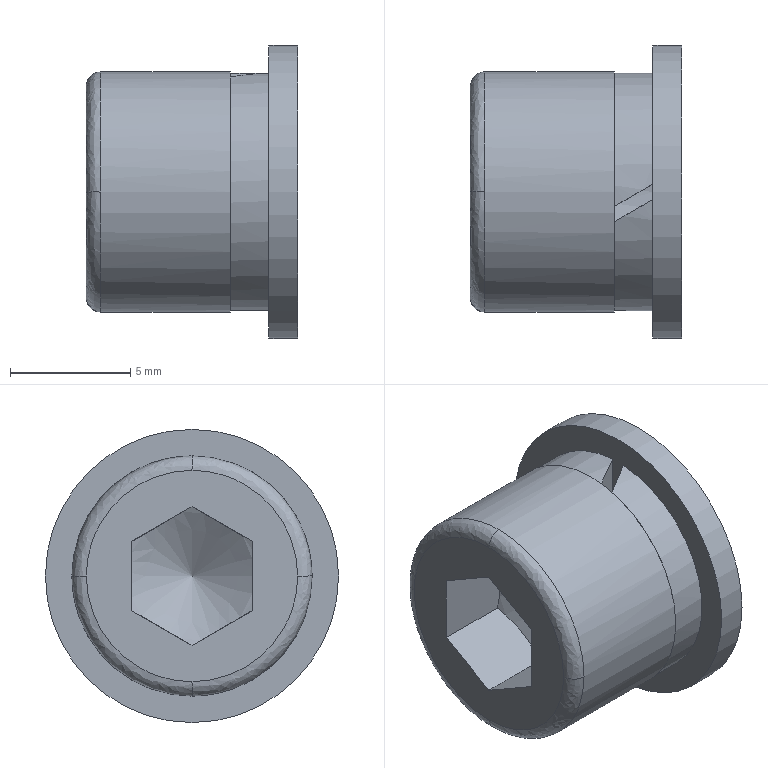Part | NX | features BREP 2 | 2 solids | 23 faces | box 8.8 x 12.2 x 12.2 mm | volume 563.29 mm3 | plane 13 | cylinder 5 | spline 4 | cone 1 | commonest cylinder face diameters 6.1 x1 6.5 x1 9.9 x1 10 x1 12.2 x1
STEP:
#1=CARTESIAN_POINT('',(96.982,177.189,-1.445));
#2=VERTEX_POINT('',#1);
#3=CARTESIAN_POINT('',(96.982,177.189,1.445));
#4=VERTEX_POINT('',#3);
#5=CARTESIAN_POINT('',(96.982,177.189,-1.445));
#6=CARTESIAN_POINT('',(97.255,177.189,-0.5008));
#7=CARTESIAN_POINT('',(97.255,177.189,0.5008));
#8=CARTESIAN_POINT('',(96.982,177.189,1.445));
#9=B_SPLINE_CURVE_WITH_KNOTS('',3,(#5,#6,#7,#8),.UNSPECIFIED.,.F.,.F.,(4,4),(0.,0.002924),.UNSPECIFIED.);
#10=EDGE_CURVE('',#2,#4,#9,.T.);
#11=ORIENTED_EDGE('',*,*,#10,.T.);
#12=CARTESIAN_POINT('',(96.982,179.689,2.887));
#13=VERTEX_POINT('',#12);
#14=CARTESIAN_POINT('',(96.982,177.189,1.445));
#15=CARTESIAN_POINT('',(97.254,178.005,1.916));
#16=CARTESIAN_POINT('',(97.254,178.872,2.416));
#17=CARTESIAN_POINT('',(96.982,179.689,2.887));
#18=B_SPLINE_CURVE_WITH_KNOTS('',3,(#14,#15,#16,#17),.UNSPECIFIED.,.F.,.F.,(4,4),(0.,0.002915),.UNSPECIFIED.);
#19=EDGE_CURVE('',#4,#13,#18,.T.);
#20=ORIENTED_EDGE('',*,*,#19,.T.);
#21=CARTESIAN_POINT('',(96.982,182.189,1.445));
#22=VERTEX_POINT('',#21);
#23=CARTESIAN_POINT('',(96.982,179.689,2.887));
#24=CARTESIAN_POINT('',(97.254,180.505,2.416));
#25=CARTESIAN_POINT('',(97.254,181.372,1.917));
#26=CARTESIAN_POINT('',(96.982,182.189,1.445));
#27=B_SPLINE_CURVE_WITH_KNOTS('',3,(#23,#24,#25,#26),.UNSPECIFIED.,.F.,.F.,(4,4),(0.,0.002915),.UNSPECIFIED.);
#28=EDGE_CURVE('',#13,#22,#27,.T.);
#29=ORIENTED_EDGE('',*,*,#28,.T.);
#30=CARTESIAN_POINT('',(96.982,182.189,-1.445));
#31=VERTEX_POINT('',#30);
#32=CARTESIAN_POINT('',(96.982,182.189,1.445));
#33=CARTESIAN_POINT('',(97.255,182.189,0.5008));
#34=CARTESIAN_POINT('',(97.255,182.189,-0.5008));
#35=CARTESIAN_POINT('',(96.982,182.189,-1.445));
#36=B_SPLINE_CURVE_WITH_KNOTS('',3,(#32,#33,#34,#35),.UNSPECIFIED.,.F.,.F.,(4,4),(0.,0.002924),.UNSPECIFIED.);
#37=EDGE_CURVE('',#22,#31,#36,.T.);
#38=ORIENTED_EDGE('',*,*,#37,.T.);
#39=CARTESIAN_POINT('',(96.982,179.689,-2.887));
#40=VERTEX_POINT('',#39);
#41=CARTESIAN_POINT('',(96.982,182.189,-1.445));
#42=CARTESIAN_POINT('',(97.254,181.373,-1.916));
#43=CARTESIAN_POINT('',(97.254,180.507,-2.416));
#44=CARTESIAN_POINT('',(96.982,179.689,-2.887));
#45=B_SPLINE_CURVE_WITH_KNOTS('',3,(#41,#42,#43,#44),.UNSPECIFIED.,.F.,.F.,(4,4),(0.,0.002915),.UNSPECIFIED.);
#46=EDGE_CURVE('',#31,#40,#45,.T.);
#47=ORIENTED_EDGE('',*,*,#46,.T.);
#48=CARTESIAN_POINT('',(96.982,179.689,-2.887));
#49=CARTESIAN_POINT('',(97.254,178.873,-2.416));
#50=CARTESIAN_POINT('',(97.254,178.007,-1.917));
#51=CARTESIAN_POINT('',(96.982,177.189,-1.445));
#52=B_SPLINE_CURVE_WITH_KNOTS('',3,(#48,#49,#50,#51),.UNSPECIFIED.,.F.,.F.,(4,4),(0.,0.002915),.UNSPECIFIED.);
#53=EDGE_CURVE('',#40,#2,#52,.T.);
#54=ORIENTED_EDGE('',*,*,#53,.T.);
#55=EDGE_LOOP('',(#11,#20,#29,#38,#47,#54));
#56=FACE_BOUND('',#55,.T.);
#57=CARTESIAN_POINT('',(98.649,179.689,0.));
#58=VERTEX_POINT('',#57);
#59=VERTEX_LOOP('',#58);
#60=FACE_BOUND('',#59,.T.);
#61=CARTESIAN_POINT('',(97.816,179.689,0.));
#62=DIRECTION('',(-1.,0.,0.));
#63=DIRECTION('',(0.,-1.,0.));
#64=AXIS2_PLACEMENT_3D('',#61,#62,#63);
#65=CONICAL_SURFACE('',#64,1.444,1.047);
#66=ADVANCED_FACE('',(#56,#60),#65,.F.);
#67=ORIENTED_EDGE('',*,*,#37,.F.);
#68=CARTESIAN_POINT('',(93.982,182.189,1.445));
#69=VERTEX_POINT('',#68);
#70=CARTESIAN_POINT('',(93.982,182.189,1.445));
#71=DIRECTION('',(1.,0.,0.));
#72=VECTOR('',#71,1000.);
#73=LINE('',#70,#72);
#74=EDGE_CURVE('',#69,#22,#73,.T.);
#75=ORIENTED_EDGE('',*,*,#74,.F.);
#76=CARTESIAN_POINT('',(93.982,182.189,-1.445));
#77=VERTEX_POINT('',#76);
#78=CARTESIAN_POINT('',(93.982,182.189,0.));
#79=DIRECTION('',(0.,0.,1.));
#80=VECTOR('',#79,1000.);
#81=LINE('',#78,#80);
#82=EDGE_CURVE('',#77,#69,#81,.T.);
#83=ORIENTED_EDGE('',*,*,#82,.F.);
#84=CARTESIAN_POINT('',(93.982,182.189,-1.445));
#85=DIRECTION('',(1.,0.,0.));
#86=VECTOR('',#85,1000.);
#87=LINE('',#84,#86);
#88=EDGE_CURVE('',#77,#31,#87,.T.);
#89=ORIENTED_EDGE('',*,*,#88,.T.);
#90=EDGE_LOOP('',(#67,#75,#83,#89));
#91=FACE_BOUND('',#90,.T.);
#92=CARTESIAN_POINT('',(93.982,182.189,-1.445));
#93=DIRECTION('',(0.,-1.,0.));
#94=DIRECTION('',(0.,0.,-1.));
#95=AXIS2_PLACEMENT_3D('',#92,#93,#94);
#96=PLANE('',#95);
#97=ADVANCED_FACE('',(#91),#96,.T.);
#98=ORIENTED_EDGE('',*,*,#46,.F.);
#99=ORIENTED_EDGE('',*,*,#88,.F.);
#100=CARTESIAN_POINT('',(93.982,179.689,-2.887));
#101=VERTEX_POINT('',#100);
#102=CARTESIAN_POINT('',(93.982,183.898,-0.4589));
#103=DIRECTION('',(0.,0.8661,0.4998));
#104=VECTOR('',#103,1000.);
#105=LINE('',#102,#104);
#106=EDGE_CURVE('',#101,#77,#105,.T.);
#107=ORIENTED_EDGE('',*,*,#106,.F.);
#108=CARTESIAN_POINT('',(93.982,179.689,-2.887));
#109=DIRECTION('',(-1.,0.,0.));
#110=VECTOR('',#109,1000.);
#111=LINE('',#108,#110);
#112=EDGE_CURVE('',#40,#101,#111,.T.);
#113=ORIENTED_EDGE('',*,*,#112,.F.);
#114=EDGE_LOOP('',(#98,#99,#107,#113));
#115=FACE_BOUND('',#114,.T.);
#116=CARTESIAN_POINT('',(93.982,179.689,-2.888));
#117=DIRECTION('',(0.,-0.4998,0.8661));
#118=DIRECTION('',(1.,0.,0.));
#119=AXIS2_PLACEMENT_3D('',#116,#117,#118);
#120=PLANE('',#119);
#121=ADVANCED_FACE('',(#115),#120,.T.);
#122=ORIENTED_EDGE('',*,*,#53,.F.);
#123=ORIENTED_EDGE('',*,*,#112,.T.);
#124=CARTESIAN_POINT('',(93.982,177.189,-1.445));
#125=VERTEX_POINT('',#124);
#126=CARTESIAN_POINT('',(93.982,181.398,-3.873));
#127=DIRECTION('',(0.,0.8661,-0.4998));
#128=VECTOR('',#127,1000.);
#129=LINE('',#126,#128);
#130=EDGE_CURVE('',#125,#101,#129,.T.);
#131=ORIENTED_EDGE('',*,*,#130,.F.);
#132=CARTESIAN_POINT('',(93.982,177.189,-1.445));
#133=DIRECTION('',(1.,0.,0.));
#134=VECTOR('',#133,1000.);
#135=LINE('',#132,#134);
#136=EDGE_CURVE('',#125,#2,#135,.T.);
#137=ORIENTED_EDGE('',*,*,#136,.T.);
#138=EDGE_LOOP('',(#122,#123,#131,#137));
#139=FACE_BOUND('',#138,.T.);
#140=CARTESIAN_POINT('',(93.982,177.189,-1.445));
#141=DIRECTION('',(0.,0.4998,0.8661));
#142=DIRECTION('',(1.,0.,0.));
#143=AXIS2_PLACEMENT_3D('',#140,#141,#142);
#144=PLANE('',#143);
#145=ADVANCED_FACE('',(#139),#144,.T.);
#146=ORIENTED_EDGE('',*,*,#10,.F.);
#147=ORIENTED_EDGE('',*,*,#136,.F.);
#148=CARTESIAN_POINT('',(93.982,177.189,1.445));
#149=VERTEX_POINT('',#148);
#150=CARTESIAN_POINT('',(93.982,177.189,0.));
#151=DIRECTION('',(0.,0.,-1.));
#152=VECTOR('',#151,1000.);
#153=LINE('',#150,#152);
#154=EDGE_CURVE('',#149,#125,#153,.T.);
#155=ORIENTED_EDGE('',*,*,#154,.F.);
#156=CARTESIAN_POINT('',(93.982,177.189,1.445));
#157=DIRECTION('',(1.,0.,0.));
#158=VECTOR('',#157,1000.);
#159=LINE('',#156,#158);
#160=EDGE_CURVE('',#149,#4,#159,.T.);
#161=ORIENTED_EDGE('',*,*,#160,.T.);
#162=EDGE_LOOP('',(#146,#147,#155,#161));
#163=FACE_BOUND('',#162,.T.);
#164=CARTESIAN_POINT('',(93.982,177.189,1.445));
#165=DIRECTION('',(0.,1.,0.));
#166=DIRECTION('',(0.,0.,1.));
#167=AXIS2_PLACEMENT_3D('',#164,#165,#166);
#168=PLANE('',#167);
#169=ADVANCED_FACE('',(#163),#168,.T.);
#170=ORIENTED_EDGE('',*,*,#19,.F.);
#171=ORIENTED_EDGE('',*,*,#160,.F.);
#172=CARTESIAN_POINT('',(93.982,179.689,2.887));
#173=VERTEX_POINT('',#172);
#174=CARTESIAN_POINT('',(93.982,181.398,3.873));
#175=DIRECTION('',(0.,-0.8661,-0.4998));
#176=VECTOR('',#175,1000.);
#177=LINE('',#174,#176);
#178=EDGE_CURVE('',#173,#149,#177,.T.);
#179=ORIENTED_EDGE('',*,*,#178,.F.);
#180=CARTESIAN_POINT('',(93.982,179.689,2.887));
#181=DIRECTION('',(1.,0.,0.));
#182=VECTOR('',#181,1000.);
#183=LINE('',#180,#182);
#184=EDGE_CURVE('',#173,#13,#183,.T.);
#185=ORIENTED_EDGE('',*,*,#184,.T.);
#186=EDGE_LOOP('',(#170,#171,#179,#185));
#187=FACE_BOUND('',#186,.T.);
#188=CARTESIAN_POINT('',(93.982,179.689,2.888));
#189=DIRECTION('',(0.,0.4998,-0.8661));
#190=DIRECTION('',(-1.,0.,0.));
#191=AXIS2_PLACEMENT_3D('',#188,#189,#190);
#192=PLANE('',#191);
#193=ADVANCED_FACE('',(#187),#192,.T.);
#194=ORIENTED_EDGE('',*,*,#28,.F.);
#195=ORIENTED_EDGE('',*,*,#184,.F.);
#196=CARTESIAN_POINT('',(93.982,183.898,0.4589));
#197=DIRECTION('',(0.,-0.8661,0.4998));
#198=VECTOR('',#197,1000.);
#199=LINE('',#196,#198);
#200=EDGE_CURVE('',#69,#173,#199,.T.);
#201=ORIENTED_EDGE('',*,*,#200,.F.);
#202=ORIENTED_EDGE('',*,*,#74,.T.);
#203=EDGE_LOOP('',(#194,#195,#201,#202));
#204=FACE_BOUND('',#203,.T.);
#205=CARTESIAN_POINT('',(93.982,182.189,1.445));
#206=DIRECTION('',(0.,-0.4998,-0.8661));
#207=DIRECTION('',(-1.,0.,0.));
#208=AXIS2_PLACEMENT_3D('',#205,#206,#207);
#209=PLANE('',#208);
#210=ADVANCED_FACE('',(#204),#209,.T.);
#211=ORIENTED_EDGE('',*,*,#200,.T.);
#212=ORIENTED_EDGE('',*,*,#178,.T.);
#213=ORIENTED_EDGE('',*,*,#154,.T.);
#214=ORIENTED_EDGE('',*,*,#130,.T.);
#215=ORIENTED_EDGE('',*,*,#106,.T.);
#216=ORIENTED_EDGE('',*,*,#82,.T.);
#217=EDGE_LOOP('',(#211,#212,#213,#214,#215,#216));
#218=FACE_BOUND('',#217,.T.);
#219=CARTESIAN_POINT('',(93.982,184.089,0.));
#220=VERTEX_POINT('',#219);
#221=CARTESIAN_POINT('',(93.982,179.689,-4.4));
#222=VERTEX_POINT('',#221);
#223=CARTESIAN_POINT('',(93.982,184.089,0.));
#224=CARTESIAN_POINT('',(93.982,184.089,-1.152));
#225=CARTESIAN_POINT('',(93.982,183.136,-3.446));
#226=CARTESIAN_POINT('',(93.982,180.841,-4.4));
#227=CARTESIAN_POINT('',(93.982,179.689,-4.4));
#228=B_SPLINE_CURVE_WITH_KNOTS('',3,(#223,#224,#225,#226,#227),.UNSPECIFIED.,.F.,.F.,(4,1,4),(0.,4.897,9.794),.UNSPECIFIED.);
#229=EDGE_CURVE('',#220,#222,#228,.T.);
#230=ORIENTED_EDGE('',*,*,#229,.T.);
#231=CARTESIAN_POINT('',(93.982,175.289,0.));
#232=VERTEX_POINT('',#231);
#233=CARTESIAN_POINT('',(93.982,179.689,-4.4));
#234=CARTESIAN_POINT('',(93.982,178.537,-4.4));
#235=CARTESIAN_POINT('',(93.982,176.243,-3.447));
#236=CARTESIAN_POINT('',(93.982,175.289,-1.152));
#237=CARTESIAN_POINT('',(93.982,175.289,0.));
#238=B_SPLINE_CURVE_WITH_KNOTS('',3,(#233,#234,#235,#236,#237),.UNSPECIFIED.,.F.,.F.,(4,1,4),(0.,4.897,9.794),.UNSPECIFIED.);
#239=EDGE_CURVE('',#222,#232,#238,.T.);
#240=ORIENTED_EDGE('',*,*,#239,.T.);
#241=CARTESIAN_POINT('',(93.982,179.689,4.4));
#242=VERTEX_POINT('',#241);
#243=CARTESIAN_POINT('',(93.982,175.289,0.));
#244=CARTESIAN_POINT('',(93.982,175.289,1.152));
#245=CARTESIAN_POINT('',(93.982,176.242,3.446));
#246=CARTESIAN_POINT('',(93.982,178.537,4.4));
#247=CARTESIAN_POINT('',(93.982,179.689,4.4));
#248=B_SPLINE_CURVE_WITH_KNOTS('',3,(#243,#244,#245,#246,#247),.UNSPECIFIED.,.F.,.F.,(4,1,4),(0.,4.896,9.791),.UNSPECIFIED.);
#249=EDGE_CURVE('',#232,#242,#248,.T.);
#250=ORIENTED_EDGE('',*,*,#249,.T.);
#251=CARTESIAN_POINT('',(93.982,179.689,4.4));
#252=CARTESIAN_POINT('',(93.982,180.841,4.4));
#253=CARTESIAN_POINT('',(93.982,183.135,3.447));
#254=CARTESIAN_POINT('',(93.982,184.089,1.152));
#255=CARTESIAN_POINT('',(93.982,184.089,0.));
#256=B_SPLINE_CURVE_WITH_KNOTS('',3,(#251,#252,#253,#254,#255),.UNSPECIFIED.,.F.,.F.,(4,1,4),(0.,4.897,9.794),.UNSPECIFIED.);
#257=EDGE_CURVE('',#242,#220,#256,.T.);
#258=ORIENTED_EDGE('',*,*,#257,.T.);
#259=EDGE_LOOP('',(#230,#240,#250,#258));
#260=FACE_BOUND('',#259,.T.);
#261=CARTESIAN_POINT('',(93.982,183.633,0.));
#262=DIRECTION('',(-1.,0.,0.));
#263=DIRECTION('',(0.,0.,1.));
#264=AXIS2_PLACEMENT_3D('',#261,#262,#263);
#265=PLANE('',#264);
#266=ADVANCED_FACE('',(#218,#260),#265,.T.);
#267=CARTESIAN_POINT('',(94.582,184.689,0.));
#268=VERTEX_POINT('',#267);
#269=CARTESIAN_POINT('',(94.582,179.689,-5.));
#270=VERTEX_POINT('',#269);
#271=CARTESIAN_POINT('',(94.582,179.689,-5.));
#272=CARTESIAN_POINT('',(94.582,180.998,-5.));
#273=CARTESIAN_POINT('',(94.582,183.606,-3.917));
#274=CARTESIAN_POINT('',(94.582,184.689,-1.309));
#275=CARTESIAN_POINT('',(94.582,184.689,0.));
#276=B_SPLINE_CURVE_WITH_KNOTS('',3,(#271,#272,#273,#274,#275),.UNSPECIFIED.,.F.,.F.,(4,1,4),(0.,0.5,1.),.UNSPECIFIED.);
#277=EDGE_CURVE('',#268,#270,#276,.F.);
#278=ORIENTED_EDGE('',*,*,#277,.T.);
#279=CARTESIAN_POINT('',(94.582,179.689,-5.));
#280=CARTESIAN_POINT('',(94.441,179.689,-5.));
#281=CARTESIAN_POINT('',(94.104,179.689,-4.878));
#282=CARTESIAN_POINT('',(93.982,179.689,-4.541));
#283=CARTESIAN_POINT('',(93.982,179.689,-4.4));
#284=B_SPLINE_CURVE_WITH_KNOTS('',3,(#279,#280,#281,#282,#283),.UNSPECIFIED.,.F.,.F.,(4,1,4),(0.,0.6414,1.283),.UNSPECIFIED.);
#285=EDGE_CURVE('',#270,#222,#284,.T.);
#286=ORIENTED_EDGE('',*,*,#285,.T.);
#287=ORIENTED_EDGE('',*,*,#229,.F.);
#288=CARTESIAN_POINT('',(93.982,184.089,0.));
#289=CARTESIAN_POINT('',(93.982,184.23,0.));
#290=CARTESIAN_POINT('',(94.104,184.567,0.));
#291=CARTESIAN_POINT('',(94.441,184.689,0.));
#292=CARTESIAN_POINT('',(94.582,184.689,0.));
#293=B_SPLINE_CURVE_WITH_KNOTS('',3,(#288,#289,#290,#291,#292),.UNSPECIFIED.,.F.,.F.,(4,1,4),(0.,0.6414,1.283),.UNSPECIFIED.);
#294=EDGE_CURVE('',#268,#220,#293,.F.);
#295=ORIENTED_EDGE('',*,*,#294,.F.);
#296=EDGE_LOOP('',(#278,#286,#287,#295));
#297=FACE_BOUND('',#296,.T.);
#298=CARTESIAN_POINT('',(94.582,184.689,0.));
#299=CARTESIAN_POINT('',(94.582,184.689,-5.));
#300=CARTESIAN_POINT('',(94.582,179.689,-5.));
#301=CARTESIAN_POINT('',(93.982,184.689,0.));
#302=CARTESIAN_POINT('',(93.982,184.689,-5.));
#303=CARTESIAN_POINT('',(93.982,179.689,-5.));
#304=CARTESIAN_POINT('',(93.982,184.089,0.));
#305=CARTESIAN_POINT('',(93.982,184.089,-4.4));
#306=CARTESIAN_POINT('',(93.982,179.689,-4.4));
#307=(BOUNDED_SURFACE()B_SPLINE_SURFACE(2,2,((#298,#299,#300),(#301,#302,#303),(#304,#305,#306)),.TOROIDAL_SURF.,.F.,.F.,.F.)B_SPLINE_SURFACE_WITH_KNOTS((3,3),(3,3),(0.,1.283),(26.4,36.),.PIECEWISE_BEZIER_KNOTS.)GEOMETRIC_REPRESENTATION_ITEM()RATIONAL_B_SPLINE_SURFACE(((1.,0.7071,1.),(0.7071,0.5,0.7071),(1.,0.7071,1.)))REPRESENTATION_ITEM('')SURFACE());
#308=ADVANCED_FACE('',(#297),#307,.F.);
#309=ORIENTED_EDGE('',*,*,#239,.F.);
#310=ORIENTED_EDGE('',*,*,#285,.F.);
#311=CARTESIAN_POINT('',(94.582,174.689,0.));
#312=VERTEX_POINT('',#311);
#313=CARTESIAN_POINT('',(94.582,174.689,0.));
#314=CARTESIAN_POINT('',(94.582,174.689,-1.309));
#315=CARTESIAN_POINT('',(94.582,175.772,-3.917));
#316=CARTESIAN_POINT('',(94.582,178.38,-5.));
#317=CARTESIAN_POINT('',(94.582,179.689,-5.));
#318=B_SPLINE_CURVE_WITH_KNOTS('',3,(#313,#314,#315,#316,#317),.UNSPECIFIED.,.F.,.F.,(4,1,4),(0.,0.5,1.),.UNSPECIFIED.);
#319=EDGE_CURVE('',#270,#312,#318,.F.);
#320=ORIENTED_EDGE('',*,*,#319,.T.);
#321=CARTESIAN_POINT('',(94.582,174.689,0.));
#322=CARTESIAN_POINT('',(94.441,174.689,0.));
#323=CARTESIAN_POINT('',(94.104,174.811,0.));
#324=CARTESIAN_POINT('',(93.982,175.148,0.));
#325=CARTESIAN_POINT('',(93.982,175.289,0.));
#326=B_SPLINE_CURVE_WITH_KNOTS('',3,(#321,#322,#323,#324,#325),.UNSPECIFIED.,.F.,.F.,(4,1,4),(0.,0.6414,1.283),.UNSPECIFIED.);
#327=EDGE_CURVE('',#312,#232,#326,.T.);
#328=ORIENTED_EDGE('',*,*,#327,.T.);
#329=EDGE_LOOP('',(#309,#310,#320,#328));
#330=FACE_BOUND('',#329,.T.);
#331=CARTESIAN_POINT('',(94.582,179.689,-5.));
#332=CARTESIAN_POINT('',(94.582,174.689,-5.));
#333=CARTESIAN_POINT('',(94.582,174.689,0.));
#334=CARTESIAN_POINT('',(93.982,179.689,-5.));
#335=CARTESIAN_POINT('',(93.982,174.689,-5.));
#336=CARTESIAN_POINT('',(93.982,174.689,0.));
#337=CARTESIAN_POINT('',(93.982,179.689,-4.4));
#338=CARTESIAN_POINT('',(93.982,175.289,-4.4));
#339=CARTESIAN_POINT('',(93.982,175.289,0.));
#340=(BOUNDED_SURFACE()B_SPLINE_SURFACE(2,2,((#331,#332,#333),(#334,#335,#336),(#337,#338,#339)),.TOROIDAL_SURF.,.F.,.F.,.F.)B_SPLINE_SURFACE_WITH_KNOTS((3,3),(3,3),(0.,1.283),(0.,9.6),.PIECEWISE_BEZIER_KNOTS.)GEOMETRIC_REPRESENTATION_ITEM()RATIONAL_B_SPLINE_SURFACE(((1.,0.7071,1.),(0.7071,0.5,0.7071),(1.,0.7071,1.)))REPRESENTATION_ITEM('')SURFACE());
#341=ADVANCED_FACE('',(#330),#340,.F.);
#342=CARTESIAN_POINT('',(94.582,179.689,5.));
#343=VERTEX_POINT('',#342);
#344=CARTESIAN_POINT('',(94.582,179.689,5.));
#345=CARTESIAN_POINT('',(94.582,178.38,5.));
#346=CARTESIAN_POINT('',(94.582,175.772,3.917));
#347=CARTESIAN_POINT('',(94.582,174.689,1.309));
#348=CARTESIAN_POINT('',(94.582,174.689,0.));
#349=B_SPLINE_CURVE_WITH_KNOTS('',3,(#344,#345,#346,#347,#348),.UNSPECIFIED.,.F.,.F.,(4,1,4),(0.,0.5,1.),.UNSPECIFIED.);
#350=EDGE_CURVE('',#312,#343,#349,.F.);
#351=ORIENTED_EDGE('',*,*,#350,.T.);
#352=CARTESIAN_POINT('',(94.582,179.689,5.));
#353=CARTESIAN_POINT('',(94.441,179.689,5.));
#354=CARTESIAN_POINT('',(94.104,179.689,4.878));
#355=CARTESIAN_POINT('',(93.982,179.689,4.541));
#356=CARTESIAN_POINT('',(93.982,179.689,4.4));
#357=B_SPLINE_CURVE_WITH_KNOTS('',3,(#352,#353,#354,#355,#356),.UNSPECIFIED.,.F.,.F.,(4,1,4),(0.,0.6414,1.283),.UNSPECIFIED.);
#358=EDGE_CURVE('',#343,#242,#357,.T.);
#359=ORIENTED_EDGE('',*,*,#358,.T.);
#360=ORIENTED_EDGE('',*,*,#249,.F.);
#361=ORIENTED_EDGE('',*,*,#327,.F.);
#362=EDGE_LOOP('',(#351,#359,#360,#361));
#363=FACE_BOUND('',#362,.T.);
#364=CARTESIAN_POINT('',(94.582,174.689,0.));
#365=CARTESIAN_POINT('',(94.582,174.689,5.));
#366=CARTESIAN_POINT('',(94.582,179.689,5.));
#367=CARTESIAN_POINT('',(93.982,174.689,0.));
#368=CARTESIAN_POINT('',(93.982,174.689,5.));
#369=CARTESIAN_POINT('',(93.982,179.689,5.));
#370=CARTESIAN_POINT('',(93.982,175.289,0.));
#371=CARTESIAN_POINT('',(93.982,175.289,4.4));
#372=CARTESIAN_POINT('',(93.982,179.689,4.4));
#373=(BOUNDED_SURFACE()B_SPLINE_SURFACE(2,2,((#364,#365,#366),(#367,#368,#369),(#370,#371,#372)),.TOROIDAL_SURF.,.F.,.F.,.F.)B_SPLINE_SURFACE_WITH_KNOTS((3,3),(3,3),(0.,1.283),(8.8,18.4),.PIECEWISE_BEZIER_KNOTS.)GEOMETRIC_REPRESENTATION_ITEM()RATIONAL_B_SPLINE_SURFACE(((1.,0.7071,1.),(0.7071,0.5,0.7071),(1.,0.7071,1.)))REPRESENTATION_ITEM('')SURFACE());
#374=ADVANCED_FACE('',(#363),#373,.F.);
#375=ORIENTED_EDGE('',*,*,#257,.F.);
#376=ORIENTED_EDGE('',*,*,#358,.F.);
#377=CARTESIAN_POINT('',(94.582,184.689,0.));
#378=CARTESIAN_POINT('',(94.582,184.689,1.309));
#379=CARTESIAN_POINT('',(94.582,183.606,3.917));
#380=CARTESIAN_POINT('',(94.582,180.998,5.));
#381=CARTESIAN_POINT('',(94.582,179.689,5.));
#382=B_SPLINE_CURVE_WITH_KNOTS('',3,(#377,#378,#379,#380,#381),.UNSPECIFIED.,.F.,.F.,(4,1,4),(0.,0.5,1.),.UNSPECIFIED.);
#383=EDGE_CURVE('',#343,#268,#382,.F.);
#384=ORIENTED_EDGE('',*,*,#383,.T.);
#385=ORIENTED_EDGE('',*,*,#294,.T.);
#386=EDGE_LOOP('',(#375,#376,#384,#385));
#387=FACE_BOUND('',#386,.T.);
#388=CARTESIAN_POINT('',(94.582,179.689,5.));
#389=CARTESIAN_POINT('',(94.582,184.689,5.));
#390=CARTESIAN_POINT('',(94.582,184.689,0.));
#391=CARTESIAN_POINT('',(93.982,179.689,5.));
#392=CARTESIAN_POINT('',(93.982,184.689,5.));
#393=CARTESIAN_POINT('',(93.982,184.689,0.));
#394=CARTESIAN_POINT('',(93.982,179.689,4.4));
#395=CARTESIAN_POINT('',(93.982,184.089,4.4));
#396=CARTESIAN_POINT('',(93.982,184.089,0.));
#397=(BOUNDED_SURFACE()B_SPLINE_SURFACE(2,2,((#388,#389,#390),(#391,#392,#393),(#394,#395,#396)),.TOROIDAL_SURF.,.F.,.F.,.F.)B_SPLINE_SURFACE_WITH_KNOTS((3,3),(3,3),(0.,1.283),(17.6,27.2),.PIECEWISE_BEZIER_KNOTS.)GEOMETRIC_REPRESENTATION_ITEM()RATIONAL_B_SPLINE_SURFACE(((1.,0.7071,1.),(0.7071,0.5,0.7071),(1.,0.7071,1.)))REPRESENTATION_ITEM('')SURFACE());
#398=ADVANCED_FACE('',(#387),#397,.F.);
#399=ORIENTED_EDGE('',*,*,#277,.F.);
#400=ORIENTED_EDGE('',*,*,#383,.F.);
#401=ORIENTED_EDGE('',*,*,#350,.F.);
#402=ORIENTED_EDGE('',*,*,#319,.F.);
#403=EDGE_LOOP('',(#399,#400,#401,#402));
#404=FACE_BOUND('',#403,.T.);
#405=CARTESIAN_POINT('',(99.982,179.689,-5.));
#406=VERTEX_POINT('',#405);
#407=CARTESIAN_POINT('',(99.982,179.689,0.));
#408=DIRECTION('',(1.,0.,0.));
#409=DIRECTION('',(0.,0.,-1.));
#410=AXIS2_PLACEMENT_3D('',#407,#408,#409);
#411=CIRCLE('',#410,5.);
#412=EDGE_CURVE('',#406,#406,#411,.F.);
#413=ORIENTED_EDGE('',*,*,#412,.T.);
#414=EDGE_LOOP('',(#413));
#415=FACE_BOUND('',#414,.T.);
#416=CARTESIAN_POINT('',(96.982,179.689,0.));
#417=DIRECTION('',(-1.,0.,0.));
#418=DIRECTION('',(0.,-1.,0.));
#419=AXIS2_PLACEMENT_3D('',#416,#417,#418);
#420=CYLINDRICAL_SURFACE('',#419,5.);
#421=ADVANCED_FACE('',(#404,#415),#420,.T.);
#422=CARTESIAN_POINT('',(99.982,178.445,3.003));
#423=VERTEX_POINT('',#422);
#424=CARTESIAN_POINT('',(99.982,179.085,3.193));
#425=VERTEX_POINT('',#424);
#426=CARTESIAN_POINT('',(99.982,179.689,0.));
#427=DIRECTION('',(1.,0.,0.));
#428=DIRECTION('',(0.,0.,-1.));
#429=AXIS2_PLACEMENT_3D('',#426,#427,#428);
#430=CIRCLE('',#429,3.25);
#431=EDGE_CURVE('',#423,#425,#430,.T.);
#432=ORIENTED_EDGE('',*,*,#431,.T.);
#433=CARTESIAN_POINT('',(99.982,179.085,4.913));
#434=VERTEX_POINT('',#433);
#435=CARTESIAN_POINT('',(99.982,179.085,0.));
#436=DIRECTION('',(0.,0.,1.));
#437=VECTOR('',#436,1000.);
#438=LINE('',#435,#437);
#439=EDGE_CURVE('',#425,#434,#438,.T.);
#440=ORIENTED_EDGE('',*,*,#439,.T.);
#441=CARTESIAN_POINT('',(99.982,178.445,4.791));
#442=VERTEX_POINT('',#441);
#443=CARTESIAN_POINT('',(99.982,179.689,0.));
#444=DIRECTION('',(1.,0.,0.));
#445=DIRECTION('',(0.,0.,-1.));
#446=AXIS2_PLACEMENT_3D('',#443,#444,#445);
#447=CIRCLE('',#446,4.95);
#448=EDGE_CURVE('',#442,#434,#447,.T.);
#449=ORIENTED_EDGE('',*,*,#448,.F.);
#450=CARTESIAN_POINT('',(99.982,178.445,0.));
#451=DIRECTION('',(0.,0.,-1.));
#452=VECTOR('',#451,1000.);
#453=LINE('',#450,#452);
#454=EDGE_CURVE('',#442,#423,#453,.T.);
#455=ORIENTED_EDGE('',*,*,#454,.T.);
#456=EDGE_LOOP('',(#432,#440,#449,#455));
#457=FACE_BOUND('',#456,.T.);
#458=ORIENTED_EDGE('',*,*,#412,.F.);
#459=EDGE_LOOP('',(#458));
#460=FACE_BOUND('',#459,.T.);
#461=CARTESIAN_POINT('',(99.982,183.689,0.));
#462=DIRECTION('',(1.,0.,0.));
#463=DIRECTION('',(0.,0.,-1.));
#464=AXIS2_PLACEMENT_3D('',#461,#462,#463);
#465=PLANE('',#464);
#466=ADVANCED_FACE('',(#457,#460),#465,.T.);
#467=ORIENTED_EDGE('',*,*,#431,.F.);
#468=CARTESIAN_POINT('',(101.582,179.369,3.234));
#469=VERTEX_POINT('',#468);
#470=CARTESIAN_POINT('',(102.136,179.689,0.));
#471=DIRECTION('',(0.5,-0.866,0.));
#472=DIRECTION('',(0.866,0.5,0.));
#473=AXIS2_PLACEMENT_3D('',#470,#471,#472);
#474=ELLIPSE('',#473,6.5,3.25);
#475=EDGE_CURVE('',#423,#469,#474,.F.);
#476=ORIENTED_EDGE('',*,*,#475,.T.);
#477=CARTESIAN_POINT('',(101.582,180.009,3.234));
#478=VERTEX_POINT('',#477);
#479=CARTESIAN_POINT('',(101.582,179.689,0.));
#480=DIRECTION('',(1.,0.,0.));
#481=DIRECTION('',(0.,0.,-1.));
#482=AXIS2_PLACEMENT_3D('',#479,#480,#481);
#483=CIRCLE('',#482,3.25);
#484=EDGE_CURVE('',#469,#478,#483,.T.);
#485=ORIENTED_EDGE('',*,*,#484,.T.);
#486=CARTESIAN_POINT('',(101.028,179.689,0.));
#487=DIRECTION('',(-0.5,0.866,0.));
#488=DIRECTION('',(0.866,0.5,0.));
#489=AXIS2_PLACEMENT_3D('',#486,#487,#488);
#490=ELLIPSE('',#489,6.5,3.25);
#491=EDGE_CURVE('',#478,#425,#490,.F.);
#492=ORIENTED_EDGE('',*,*,#491,.T.);
#493=EDGE_LOOP('',(#467,#476,#485,#492));
#494=FACE_BOUND('',#493,.T.);
#495=CARTESIAN_POINT('',(100.782,179.689,0.));
#496=DIRECTION('',(1.,0.,0.));
#497=DIRECTION('',(0.,1.,0.));
#498=AXIS2_PLACEMENT_3D('',#495,#496,#497);
#499=CYLINDRICAL_SURFACE('',#498,3.25);
#500=ADVANCED_FACE('',(#494),#499,.F.);
#501=CARTESIAN_POINT('',(101.582,180.009,4.94));
#502=VERTEX_POINT('',#501);
#503=CARTESIAN_POINT('',(101.028,179.689,0.));
#504=DIRECTION('',(-0.5,0.866,0.));
#505=DIRECTION('',(0.866,0.5,0.));
#506=AXIS2_PLACEMENT_3D('',#503,#504,#505);
#507=ELLIPSE('',#506,9.9,4.95);
#508=EDGE_CURVE('',#434,#502,#507,.T.);
#509=ORIENTED_EDGE('',*,*,#508,.F.);
#510=ORIENTED_EDGE('',*,*,#439,.F.);
#511=ORIENTED_EDGE('',*,*,#491,.F.);
#512=CARTESIAN_POINT('',(101.582,180.009,0.));
#513=DIRECTION('',(0.,0.,-1.));
#514=VECTOR('',#513,1000.);
#515=LINE('',#512,#514);
#516=EDGE_CURVE('',#502,#478,#515,.T.);
#517=ORIENTED_EDGE('',*,*,#516,.F.);
#518=EDGE_LOOP('',(#509,#510,#511,#517));
#519=FACE_BOUND('',#518,.T.);
#520=CARTESIAN_POINT('',(99.982,179.085,0.));
#521=DIRECTION('',(-0.5,0.866,0.));
#522=DIRECTION('',(0.,0.,1.));
#523=AXIS2_PLACEMENT_3D('',#520,#521,#522);
#524=PLANE('',#523);
#525=ADVANCED_FACE('',(#519),#524,.F.);
#526=CARTESIAN_POINT('',(101.582,179.369,4.94));
#527=VERTEX_POINT('',#526);
#528=CARTESIAN_POINT('',(102.136,179.689,0.));
#529=DIRECTION('',(0.5,-0.866,0.));
#530=DIRECTION('',(0.866,0.5,0.));
#531=AXIS2_PLACEMENT_3D('',#528,#529,#530);
#532=ELLIPSE('',#531,9.9,4.95);
#533=EDGE_CURVE('',#527,#442,#532,.T.);
#534=ORIENTED_EDGE('',*,*,#533,.F.);
#535=CARTESIAN_POINT('',(101.582,179.369,0.));
#536=DIRECTION('',(0.,0.,1.));
#537=VECTOR('',#536,1000.);
#538=LINE('',#535,#537);
#539=EDGE_CURVE('',#469,#527,#538,.T.);
#540=ORIENTED_EDGE('',*,*,#539,.F.);
#541=ORIENTED_EDGE('',*,*,#475,.F.);
#542=ORIENTED_EDGE('',*,*,#454,.F.);
#543=EDGE_LOOP('',(#534,#540,#541,#542));
#544=FACE_BOUND('',#543,.T.);
#545=CARTESIAN_POINT('',(101.582,179.369,0.));
#546=DIRECTION('',(0.5,-0.866,0.));
#547=DIRECTION('',(0.,0.,-1.));
#548=AXIS2_PLACEMENT_3D('',#545,#546,#547);
#549=PLANE('',#548);
#550=ADVANCED_FACE('',(#544),#549,.F.);
#551=ORIENTED_EDGE('',*,*,#516,.T.);
#552=ORIENTED_EDGE('',*,*,#484,.F.);
#553=ORIENTED_EDGE('',*,*,#539,.T.);
#554=CARTESIAN_POINT('',(101.582,179.689,0.));
#555=DIRECTION('',(1.,0.,0.));
#556=DIRECTION('',(0.,0.,-1.));
#557=AXIS2_PLACEMENT_3D('',#554,#555,#556);
#558=CIRCLE('',#557,4.95);
#559=EDGE_CURVE('',#527,#502,#558,.T.);
#560=ORIENTED_EDGE('',*,*,#559,.T.);
#561=EDGE_LOOP('',(#551,#552,#553,#560));
#562=FACE_BOUND('',#561,.T.);
#563=CARTESIAN_POINT('',(101.582,183.789,0.));
#564=DIRECTION('',(1.,0.,0.));
#565=DIRECTION('',(0.,0.,-1.));
#566=AXIS2_PLACEMENT_3D('',#563,#564,#565);
#567=PLANE('',#566);
#568=ADVANCED_FACE('',(#562),#567,.T.);
#569=ORIENTED_EDGE('',*,*,#448,.T.);
#570=ORIENTED_EDGE('',*,*,#508,.T.);
#571=ORIENTED_EDGE('',*,*,#559,.F.);
#572=ORIENTED_EDGE('',*,*,#533,.T.);
#573=EDGE_LOOP('',(#569,#570,#571,#572));
#574=FACE_BOUND('',#573,.T.);
#575=CARTESIAN_POINT('',(100.782,179.689,0.));
#576=DIRECTION('',(1.,0.,0.));
#577=DIRECTION('',(0.,1.,0.));
#578=AXIS2_PLACEMENT_3D('',#575,#576,#577);
#579=CYLINDRICAL_SURFACE('',#578,4.95);
#580=ADVANCED_FACE('',(#574),#579,.T.);
#581=CLOSED_SHELL('',(#66,#97,#121,#145,#169,#193,#210,#266,#308,#341,#374,#398,#421,#466,#500,#525,#550,#568,#580));
#582=MANIFOLD_SOLID_BREP('',#581);
#583=CARTESIAN_POINT('',(102.782,179.689,3.05));
#584=VERTEX_POINT('',#583);
#585=CARTESIAN_POINT('',(102.782,179.689,0.));
#586=DIRECTION('',(-1.,0.,0.));
#587=DIRECTION('',(0.,0.,1.));
#588=AXIS2_PLACEMENT_3D('',#585,#586,#587);
#589=CIRCLE('',#588,3.05);
#590=EDGE_CURVE('',#584,#584,#589,.T.);
#591=ORIENTED_EDGE('',*,*,#590,.T.);
#592=EDGE_LOOP('',(#591));
#593=FACE_BOUND('',#592,.T.);
#594=CARTESIAN_POINT('',(102.782,179.689,6.1));
#595=VERTEX_POINT('',#594);
#596=CARTESIAN_POINT('',(102.782,179.689,0.));
#597=DIRECTION('',(-1.,0.,0.));
#598=DIRECTION('',(0.,0.,1.));
#599=AXIS2_PLACEMENT_3D('',#596,#597,#598);
#600=CIRCLE('',#599,6.1);
#601=EDGE_CURVE('',#595,#595,#600,.T.);
#602=ORIENTED_EDGE('',*,*,#601,.F.);
#603=EDGE_LOOP('',(#602));
#604=FACE_BOUND('',#603,.T.);
#605=CARTESIAN_POINT('',(102.782,185.789,0.));
#606=DIRECTION('',(-1.,0.,0.));
#607=DIRECTION('',(0.,0.,-1.));
#608=AXIS2_PLACEMENT_3D('',#605,#606,#607);
#609=PLANE('',#608);
#610=ADVANCED_FACE('',(#593,#604),#609,.F.);
#611=CARTESIAN_POINT('',(101.582,179.689,3.05));
#612=VERTEX_POINT('',#611);
#613=CARTESIAN_POINT('',(101.582,179.689,0.));
#614=DIRECTION('',(-1.,0.,0.));
#615=DIRECTION('',(0.,0.,1.));
#616=AXIS2_PLACEMENT_3D('',#613,#614,#615);
#617=CIRCLE('',#616,3.05);
#618=EDGE_CURVE('',#612,#612,#617,.T.);
#619=ORIENTED_EDGE('',*,*,#618,.F.);
#620=EDGE_LOOP('',(#619));
#621=FACE_BOUND('',#620,.T.);
#622=CARTESIAN_POINT('',(101.582,179.689,6.1));
#623=VERTEX_POINT('',#622);
#624=CARTESIAN_POINT('',(101.582,179.689,0.));
#625=DIRECTION('',(-1.,0.,0.));
#626=DIRECTION('',(0.,0.,1.));
#627=AXIS2_PLACEMENT_3D('',#624,#625,#626);
#628=CIRCLE('',#627,6.1);
#629=EDGE_CURVE('',#623,#623,#628,.T.);
#630=ORIENTED_EDGE('',*,*,#629,.T.);
#631=EDGE_LOOP('',(#630));
#632=FACE_BOUND('',#631,.T.);
#633=CARTESIAN_POINT('',(101.582,182.739,0.));
#634=DIRECTION('',(-1.,0.,0.));
#635=DIRECTION('',(0.,0.,-1.));
#636=AXIS2_PLACEMENT_3D('',#633,#634,#635);
#637=PLANE('',#636);
#638=ADVANCED_FACE('',(#621,#632),#637,.T.);
#639=ORIENTED_EDGE('',*,*,#618,.T.);
#640=EDGE_LOOP('',(#639));
#641=FACE_BOUND('',#640,.T.);
#642=ORIENTED_EDGE('',*,*,#590,.F.);
#643=EDGE_LOOP('',(#642));
#644=FACE_BOUND('',#643,.T.);
#645=CARTESIAN_POINT('',(102.182,179.689,0.));
#646=DIRECTION('',(-1.,0.,0.));
#647=DIRECTION('',(0.,0.,-1.));
#648=AXIS2_PLACEMENT_3D('',#645,#646,#647);
#649=CYLINDRICAL_SURFACE('',#648,3.05);
#650=ADVANCED_FACE('',(#641,#644),#649,.F.);
#651=ORIENTED_EDGE('',*,*,#601,.T.);
#652=EDGE_LOOP('',(#651));
#653=FACE_BOUND('',#652,.T.);
#654=ORIENTED_EDGE('',*,*,#629,.F.);
#655=EDGE_LOOP('',(#654));
#656=FACE_BOUND('',#655,.T.);
#657=CARTESIAN_POINT('',(102.182,179.689,0.));
#658=DIRECTION('',(-1.,0.,0.));
#659=DIRECTION('',(0.,0.,-1.));
#660=AXIS2_PLACEMENT_3D('',#657,#658,#659);
#661=CYLINDRICAL_SURFACE('',#660,6.1);
#662=ADVANCED_FACE('',(#653,#656),#661,.T.);
#663=CLOSED_SHELL('',(#610,#638,#650,#662));
#664=MANIFOLD_SOLID_BREP('',#663);
#665=(LENGTH_UNIT()NAMED_UNIT(*)SI_UNIT(.MILLI.,.METRE.));
#666=UNCERTAINTY_MEASURE_WITH_UNIT(LENGTH_MEASURE(0.0508),#665,'','');
#667=(NAMED_UNIT(*)PLANE_ANGLE_UNIT()SI_UNIT($,.RADIAN.));
#668=(NAMED_UNIT(*)SI_UNIT($,.STERADIAN.)SOLID_ANGLE_UNIT());
#669=(GEOMETRIC_REPRESENTATION_CONTEXT(3)GLOBAL_UNCERTAINTY_ASSIGNED_CONTEXT((#666))GLOBAL_UNIT_ASSIGNED_CONTEXT((#665,#667,#668))REPRESENTATION_CONTEXT('',''));
#670=ADVANCED_BREP_SHAPE_REPRESENTATION('',(#582,#664),#669);